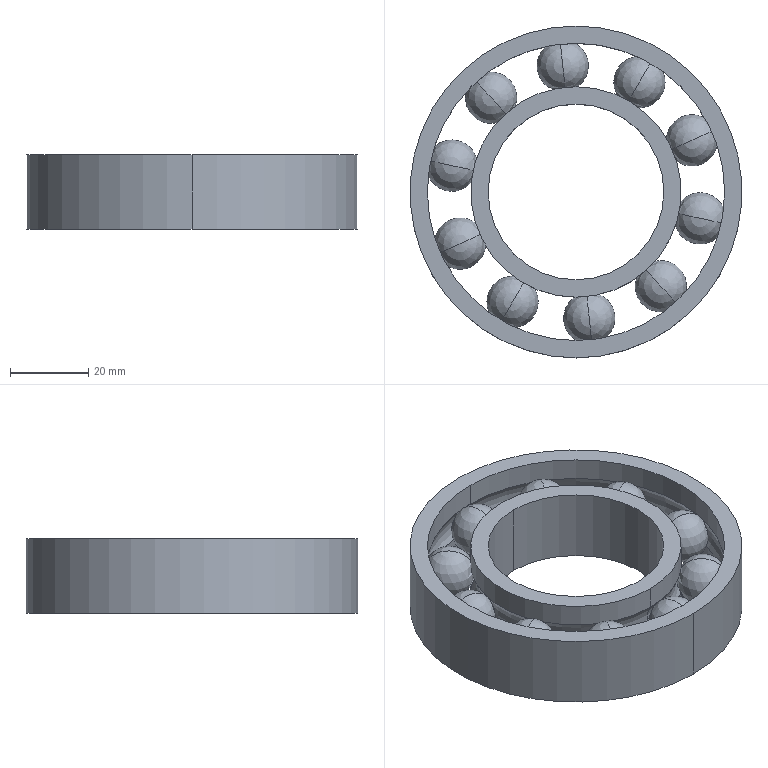Part | NX | features BREP 12 | 12 solids | 40 faces | box 85 x 85 x 19 mm | volume 44629 mm3 | sphere 20 | cylinder 12 | torus 4 | plane 4 | commonest cylinder face diameters 53.889 x4 76.111 x4 45 x2 85 x2
STEP:
#1=CARTESIAN_POINT('',(29.69,13.219,6.667));
#2=VERTEX_POINT('',#1);
#3=CARTESIAN_POINT('',(29.69,13.219,-6.667));
#4=VERTEX_POINT('',#3);
#5=CARTESIAN_POINT('',(29.69,13.219,0.));
#6=DIRECTION('',(-0.4067,0.9135,0.));
#7=DIRECTION('',(0.,0.,-1.));
#8=AXIS2_PLACEMENT_3D('',#5,#6,#7);
#9=CIRCLE('',#8,6.667);
#10=EDGE_CURVE('',#2,#4,#9,.F.);
#11=ORIENTED_EDGE('',*,*,#10,.T.);
#12=CARTESIAN_POINT('',(29.69,13.219,0.));
#13=DIRECTION('',(0.4067,-0.9135,0.));
#14=DIRECTION('',(0.,0.,-1.));
#15=AXIS2_PLACEMENT_3D('',#12,#13,#14);
#16=CIRCLE('',#15,6.667);
#17=EDGE_CURVE('',#2,#4,#16,.F.);
#18=ORIENTED_EDGE('',*,*,#17,.F.);
#19=EDGE_LOOP('',(#11,#18));
#20=FACE_BOUND('',#19,.T.);
#21=CARTESIAN_POINT('',(29.69,13.219,0.));
#22=DIRECTION('',(0.,0.,-1.));
#23=DIRECTION('',(0.9135,0.4067,0.));
#24=AXIS2_PLACEMENT_3D('',#21,#22,#23);
#25=SPHERICAL_SURFACE('',#24,6.667);
#26=ADVANCED_FACE('',(#20),#25,.T.);
#27=ORIENTED_EDGE('',*,*,#10,.F.);
#28=ORIENTED_EDGE('',*,*,#17,.T.);
#29=EDGE_LOOP('',(#27,#28));
#30=FACE_BOUND('',#29,.T.);
#31=CARTESIAN_POINT('',(29.69,13.219,0.));
#32=DIRECTION('',(0.,0.,-1.));
#33=DIRECTION('',(0.9135,0.4067,0.));
#34=AXIS2_PLACEMENT_3D('',#31,#32,#33);
#35=SPHERICAL_SURFACE('',#34,6.667);
#36=ADVANCED_FACE('',(#30),#35,.T.);
#37=CLOSED_SHELL('',(#26,#36));
#38=MANIFOLD_SOLID_BREP('',#37);
#39=CARTESIAN_POINT('',(31.79,-6.757,6.667));
#40=VERTEX_POINT('',#39);
#41=CARTESIAN_POINT('',(31.79,-6.757,-6.667));
#42=VERTEX_POINT('',#41);
#43=CARTESIAN_POINT('',(31.79,-6.757,0.));
#44=DIRECTION('',(0.2079,0.9781,0.));
#45=DIRECTION('',(0.,0.,-1.));
#46=AXIS2_PLACEMENT_3D('',#43,#44,#45);
#47=CIRCLE('',#46,6.667);
#48=EDGE_CURVE('',#40,#42,#47,.F.);
#49=ORIENTED_EDGE('',*,*,#48,.T.);
#50=CARTESIAN_POINT('',(31.79,-6.757,0.));
#51=DIRECTION('',(-0.2079,-0.9781,0.));
#52=DIRECTION('',(0.,0.,-1.));
#53=AXIS2_PLACEMENT_3D('',#50,#51,#52);
#54=CIRCLE('',#53,6.667);
#55=EDGE_CURVE('',#40,#42,#54,.F.);
#56=ORIENTED_EDGE('',*,*,#55,.F.);
#57=EDGE_LOOP('',(#49,#56));
#58=FACE_BOUND('',#57,.T.);
#59=CARTESIAN_POINT('',(31.79,-6.757,0.));
#60=DIRECTION('',(0.,0.,-1.));
#61=DIRECTION('',(0.9781,-0.2079,0.));
#62=AXIS2_PLACEMENT_3D('',#59,#60,#61);
#63=SPHERICAL_SURFACE('',#62,6.667);
#64=ADVANCED_FACE('',(#58),#63,.T.);
#65=ORIENTED_EDGE('',*,*,#48,.F.);
#66=ORIENTED_EDGE('',*,*,#55,.T.);
#67=EDGE_LOOP('',(#65,#66));
#68=FACE_BOUND('',#67,.T.);
#69=CARTESIAN_POINT('',(31.79,-6.757,0.));
#70=DIRECTION('',(0.,0.,-1.));
#71=DIRECTION('',(0.9781,-0.2079,0.));
#72=AXIS2_PLACEMENT_3D('',#69,#70,#71);
#73=SPHERICAL_SURFACE('',#72,6.667);
#74=ADVANCED_FACE('',(#68),#73,.T.);
#75=CLOSED_SHELL('',(#64,#74));
#76=MANIFOLD_SOLID_BREP('',#75);
#77=CARTESIAN_POINT('',(-16.25,-28.146,-6.667));
#78=VERTEX_POINT('',#77);
#79=CARTESIAN_POINT('',(-16.25,-28.146,6.667));
#80=VERTEX_POINT('',#79);
#81=CARTESIAN_POINT('',(-16.25,-28.146,0.));
#82=DIRECTION('',(0.866,-0.5,0.));
#83=DIRECTION('',(0.,0.,-1.));
#84=AXIS2_PLACEMENT_3D('',#81,#82,#83);
#85=CIRCLE('',#84,6.667);
#86=EDGE_CURVE('',#78,#80,#85,.T.);
#87=ORIENTED_EDGE('',*,*,#86,.F.);
#88=CARTESIAN_POINT('',(-16.25,-28.146,0.));
#89=DIRECTION('',(-0.866,0.5,0.));
#90=DIRECTION('',(0.,0.,-1.));
#91=AXIS2_PLACEMENT_3D('',#88,#89,#90);
#92=CIRCLE('',#91,6.667);
#93=EDGE_CURVE('',#78,#80,#92,.T.);
#94=ORIENTED_EDGE('',*,*,#93,.T.);
#95=EDGE_LOOP('',(#87,#94));
#96=FACE_BOUND('',#95,.T.);
#97=CARTESIAN_POINT('',(-16.25,-28.146,0.));
#98=DIRECTION('',(0.,0.,-1.));
#99=DIRECTION('',(-0.5,-0.866,0.));
#100=AXIS2_PLACEMENT_3D('',#97,#98,#99);
#101=SPHERICAL_SURFACE('',#100,6.667);
#102=ADVANCED_FACE('',(#96),#101,.T.);
#103=ORIENTED_EDGE('',*,*,#86,.T.);
#104=ORIENTED_EDGE('',*,*,#93,.F.);
#105=EDGE_LOOP('',(#103,#104));
#106=FACE_BOUND('',#105,.T.);
#107=CARTESIAN_POINT('',(-16.25,-28.146,0.));
#108=DIRECTION('',(0.,0.,-1.));
#109=DIRECTION('',(-0.5,-0.866,0.));
#110=AXIS2_PLACEMENT_3D('',#107,#108,#109);
#111=SPHERICAL_SURFACE('',#110,6.667);
#112=ADVANCED_FACE('',(#106),#111,.T.);
#113=CLOSED_SHELL('',(#102,#112));
#114=MANIFOLD_SOLID_BREP('',#113);
#115=CARTESIAN_POINT('',(16.25,28.146,6.667));
#116=VERTEX_POINT('',#115);
#117=CARTESIAN_POINT('',(16.25,28.146,-6.667));
#118=VERTEX_POINT('',#117);
#119=CARTESIAN_POINT('',(16.25,28.146,0.));
#120=DIRECTION('',(-0.866,0.5,0.));
#121=DIRECTION('',(0.,0.,-1.));
#122=AXIS2_PLACEMENT_3D('',#119,#120,#121);
#123=CIRCLE('',#122,6.667);
#124=EDGE_CURVE('',#116,#118,#123,.F.);
#125=ORIENTED_EDGE('',*,*,#124,.T.);
#126=CARTESIAN_POINT('',(16.25,28.146,0.));
#127=DIRECTION('',(0.866,-0.5,0.));
#128=DIRECTION('',(0.,0.,-1.));
#129=AXIS2_PLACEMENT_3D('',#126,#127,#128);
#130=CIRCLE('',#129,6.667);
#131=EDGE_CURVE('',#116,#118,#130,.F.);
#132=ORIENTED_EDGE('',*,*,#131,.F.);
#133=EDGE_LOOP('',(#125,#132));
#134=FACE_BOUND('',#133,.T.);
#135=CARTESIAN_POINT('',(16.25,28.146,0.));
#136=DIRECTION('',(0.,0.,-1.));
#137=DIRECTION('',(0.5,0.866,0.));
#138=AXIS2_PLACEMENT_3D('',#135,#136,#137);
#139=SPHERICAL_SURFACE('',#138,6.667);
#140=ADVANCED_FACE('',(#134),#139,.T.);
#141=ORIENTED_EDGE('',*,*,#124,.F.);
#142=ORIENTED_EDGE('',*,*,#131,.T.);
#143=EDGE_LOOP('',(#141,#142));
#144=FACE_BOUND('',#143,.T.);
#145=CARTESIAN_POINT('',(16.25,28.146,0.));
#146=DIRECTION('',(0.,0.,-1.));
#147=DIRECTION('',(0.5,0.866,0.));
#148=AXIS2_PLACEMENT_3D('',#145,#146,#147);
#149=SPHERICAL_SURFACE('',#148,6.667);
#150=ADVANCED_FACE('',(#144),#149,.T.);
#151=CLOSED_SHELL('',(#140,#150));
#152=MANIFOLD_SOLID_BREP('',#151);
#153=CARTESIAN_POINT('',(-31.79,6.757,-6.667));
#154=VERTEX_POINT('',#153);
#155=CARTESIAN_POINT('',(-31.79,6.757,6.667));
#156=VERTEX_POINT('',#155);
#157=CARTESIAN_POINT('',(-31.79,6.757,0.));
#158=DIRECTION('',(-0.2079,-0.9781,0.));
#159=DIRECTION('',(0.,0.,-1.));
#160=AXIS2_PLACEMENT_3D('',#157,#158,#159);
#161=CIRCLE('',#160,6.667);
#162=EDGE_CURVE('',#154,#156,#161,.T.);
#163=ORIENTED_EDGE('',*,*,#162,.F.);
#164=CARTESIAN_POINT('',(-31.79,6.757,0.));
#165=DIRECTION('',(0.2079,0.9781,0.));
#166=DIRECTION('',(0.,0.,-1.));
#167=AXIS2_PLACEMENT_3D('',#164,#165,#166);
#168=CIRCLE('',#167,6.667);
#169=EDGE_CURVE('',#154,#156,#168,.T.);
#170=ORIENTED_EDGE('',*,*,#169,.T.);
#171=EDGE_LOOP('',(#163,#170));
#172=FACE_BOUND('',#171,.T.);
#173=CARTESIAN_POINT('',(-31.79,6.757,0.));
#174=DIRECTION('',(0.,0.,-1.));
#175=DIRECTION('',(-0.9781,0.2079,0.));
#176=AXIS2_PLACEMENT_3D('',#173,#174,#175);
#177=SPHERICAL_SURFACE('',#176,6.667);
#178=ADVANCED_FACE('',(#172),#177,.T.);
#179=ORIENTED_EDGE('',*,*,#162,.T.);
#180=ORIENTED_EDGE('',*,*,#169,.F.);
#181=EDGE_LOOP('',(#179,#180));
#182=FACE_BOUND('',#181,.T.);
#183=CARTESIAN_POINT('',(-31.79,6.757,0.));
#184=DIRECTION('',(0.,0.,-1.));
#185=DIRECTION('',(-0.9781,0.2079,0.));
#186=AXIS2_PLACEMENT_3D('',#183,#184,#185);
#187=SPHERICAL_SURFACE('',#186,6.667);
#188=ADVANCED_FACE('',(#182),#187,.T.);
#189=CLOSED_SHELL('',(#178,#188));
#190=MANIFOLD_SOLID_BREP('',#189);
#191=CARTESIAN_POINT('',(3.397,-32.322,6.667));
#192=VERTEX_POINT('',#191);
#193=CARTESIAN_POINT('',(3.397,-32.322,-6.667));
#194=VERTEX_POINT('',#193);
#195=CARTESIAN_POINT('',(3.397,-32.322,0.));
#196=DIRECTION('',(0.9945,0.1045,0.));
#197=DIRECTION('',(0.,0.,-1.));
#198=AXIS2_PLACEMENT_3D('',#195,#196,#197);
#199=CIRCLE('',#198,6.667);
#200=EDGE_CURVE('',#192,#194,#199,.F.);
#201=ORIENTED_EDGE('',*,*,#200,.T.);
#202=CARTESIAN_POINT('',(3.397,-32.322,0.));
#203=DIRECTION('',(-0.9945,-0.1045,0.));
#204=DIRECTION('',(0.,0.,-1.));
#205=AXIS2_PLACEMENT_3D('',#202,#203,#204);
#206=CIRCLE('',#205,6.667);
#207=EDGE_CURVE('',#192,#194,#206,.F.);
#208=ORIENTED_EDGE('',*,*,#207,.F.);
#209=EDGE_LOOP('',(#201,#208));
#210=FACE_BOUND('',#209,.T.);
#211=CARTESIAN_POINT('',(3.397,-32.322,0.));
#212=DIRECTION('',(0.,0.,-1.));
#213=DIRECTION('',(0.1045,-0.9945,0.));
#214=AXIS2_PLACEMENT_3D('',#211,#212,#213);
#215=SPHERICAL_SURFACE('',#214,6.667);
#216=ADVANCED_FACE('',(#210),#215,.T.);
#217=ORIENTED_EDGE('',*,*,#200,.F.);
#218=ORIENTED_EDGE('',*,*,#207,.T.);
#219=EDGE_LOOP('',(#217,#218));
#220=FACE_BOUND('',#219,.T.);
#221=CARTESIAN_POINT('',(3.397,-32.322,0.));
#222=DIRECTION('',(0.,0.,-1.));
#223=DIRECTION('',(0.1045,-0.9945,0.));
#224=AXIS2_PLACEMENT_3D('',#221,#222,#223);
#225=SPHERICAL_SURFACE('',#224,6.667);
#226=ADVANCED_FACE('',(#220),#225,.T.);
#227=CLOSED_SHELL('',(#216,#226));
#228=MANIFOLD_SOLID_BREP('',#227);
#229=CARTESIAN_POINT('',(-29.69,-13.219,-6.667));
#230=VERTEX_POINT('',#229);
#231=CARTESIAN_POINT('',(-29.69,-13.219,6.667));
#232=VERTEX_POINT('',#231);
#233=CARTESIAN_POINT('',(-29.69,-13.219,0.));
#234=DIRECTION('',(0.4067,-0.9135,0.));
#235=DIRECTION('',(0.,0.,-1.));
#236=AXIS2_PLACEMENT_3D('',#233,#234,#235);
#237=CIRCLE('',#236,6.667);
#238=EDGE_CURVE('',#230,#232,#237,.T.);
#239=ORIENTED_EDGE('',*,*,#238,.F.);
#240=CARTESIAN_POINT('',(-29.69,-13.219,0.));
#241=DIRECTION('',(-0.4067,0.9135,0.));
#242=DIRECTION('',(0.,0.,-1.));
#243=AXIS2_PLACEMENT_3D('',#240,#241,#242);
#244=CIRCLE('',#243,6.667);
#245=EDGE_CURVE('',#230,#232,#244,.T.);
#246=ORIENTED_EDGE('',*,*,#245,.T.);
#247=EDGE_LOOP('',(#239,#246));
#248=FACE_BOUND('',#247,.T.);
#249=CARTESIAN_POINT('',(-29.69,-13.219,0.));
#250=DIRECTION('',(0.,0.,-1.));
#251=DIRECTION('',(-0.9135,-0.4067,0.));
#252=AXIS2_PLACEMENT_3D('',#249,#250,#251);
#253=SPHERICAL_SURFACE('',#252,6.667);
#254=ADVANCED_FACE('',(#248),#253,.T.);
#255=ORIENTED_EDGE('',*,*,#238,.T.);
#256=ORIENTED_EDGE('',*,*,#245,.F.);
#257=EDGE_LOOP('',(#255,#256));
#258=FACE_BOUND('',#257,.T.);
#259=CARTESIAN_POINT('',(-29.69,-13.219,0.));
#260=DIRECTION('',(0.,0.,-1.));
#261=DIRECTION('',(-0.9135,-0.4067,0.));
#262=AXIS2_PLACEMENT_3D('',#259,#260,#261);
#263=SPHERICAL_SURFACE('',#262,6.667);
#264=ADVANCED_FACE('',(#258),#263,.T.);
#265=CLOSED_SHELL('',(#254,#264));
#266=MANIFOLD_SOLID_BREP('',#265);
#267=CARTESIAN_POINT('',(-21.747,24.152,-6.667));
#268=VERTEX_POINT('',#267);
#269=CARTESIAN_POINT('',(-21.747,24.152,6.667));
#270=VERTEX_POINT('',#269);
#271=CARTESIAN_POINT('',(-21.747,24.152,0.));
#272=DIRECTION('',(-0.7431,-0.6691,0.));
#273=DIRECTION('',(0.,0.,-1.));
#274=AXIS2_PLACEMENT_3D('',#271,#272,#273);
#275=CIRCLE('',#274,6.667);
#276=EDGE_CURVE('',#268,#270,#275,.T.);
#277=ORIENTED_EDGE('',*,*,#276,.F.);
#278=CARTESIAN_POINT('',(-21.747,24.152,0.));
#279=DIRECTION('',(0.7431,0.6691,0.));
#280=DIRECTION('',(0.,0.,-1.));
#281=AXIS2_PLACEMENT_3D('',#278,#279,#280);
#282=CIRCLE('',#281,6.667);
#283=EDGE_CURVE('',#268,#270,#282,.T.);
#284=ORIENTED_EDGE('',*,*,#283,.T.);
#285=EDGE_LOOP('',(#277,#284));
#286=FACE_BOUND('',#285,.T.);
#287=CARTESIAN_POINT('',(-21.747,24.152,0.));
#288=DIRECTION('',(0.,0.,-1.));
#289=DIRECTION('',(-0.6691,0.7431,0.));
#290=AXIS2_PLACEMENT_3D('',#287,#288,#289);
#291=SPHERICAL_SURFACE('',#290,6.667);
#292=ADVANCED_FACE('',(#286),#291,.T.);
#293=ORIENTED_EDGE('',*,*,#276,.T.);
#294=ORIENTED_EDGE('',*,*,#283,.F.);
#295=EDGE_LOOP('',(#293,#294));
#296=FACE_BOUND('',#295,.T.);
#297=CARTESIAN_POINT('',(-21.747,24.152,0.));
#298=DIRECTION('',(0.,0.,-1.));
#299=DIRECTION('',(-0.6691,0.7431,0.));
#300=AXIS2_PLACEMENT_3D('',#297,#298,#299);
#301=SPHERICAL_SURFACE('',#300,6.667);
#302=ADVANCED_FACE('',(#296),#301,.T.);
#303=CLOSED_SHELL('',(#292,#302));
#304=MANIFOLD_SOLID_BREP('',#303);
#305=CARTESIAN_POINT('',(0.,26.944,3.685));
#306=VERTEX_POINT('',#305);
#307=CARTESIAN_POINT('',(0.,-26.944,3.685));
#308=VERTEX_POINT('',#307);
#309=CARTESIAN_POINT('',(0.,0.,3.685));
#310=DIRECTION('',(0.,0.,1.));
#311=DIRECTION('',(0.,1.,0.));
#312=AXIS2_PLACEMENT_3D('',#309,#310,#311);
#313=CIRCLE('',#312,26.944);
#314=EDGE_CURVE('',#306,#308,#313,.T.);
#315=ORIENTED_EDGE('',*,*,#314,.T.);
#316=CARTESIAN_POINT('',(0.,-26.944,9.5));
#317=VERTEX_POINT('',#316);
#318=CARTESIAN_POINT('',(0.,-26.944,3.685));
#319=DIRECTION('',(0.,0.,1.));
#320=VECTOR('',#319,1000.);
#321=LINE('',#318,#320);
#322=EDGE_CURVE('',#308,#317,#321,.T.);
#323=ORIENTED_EDGE('',*,*,#322,.T.);
#324=CARTESIAN_POINT('',(0.,26.944,9.5));
#325=VERTEX_POINT('',#324);
#326=CARTESIAN_POINT('',(0.,0.,9.5));
#327=DIRECTION('',(0.,0.,1.));
#328=DIRECTION('',(0.,1.,0.));
#329=AXIS2_PLACEMENT_3D('',#326,#327,#328);
#330=CIRCLE('',#329,26.944);
#331=EDGE_CURVE('',#325,#317,#330,.T.);
#332=ORIENTED_EDGE('',*,*,#331,.F.);
#333=CARTESIAN_POINT('',(0.,26.944,3.685));
#334=DIRECTION('',(0.,0.,1.));
#335=VECTOR('',#334,1000.);
#336=LINE('',#333,#335);
#337=EDGE_CURVE('',#306,#325,#336,.T.);
#338=ORIENTED_EDGE('',*,*,#337,.F.);
#339=EDGE_LOOP('',(#315,#323,#332,#338));
#340=FACE_BOUND('',#339,.T.);
#341=CARTESIAN_POINT('',(0.,0.,10.45));
#342=DIRECTION('',(0.,0.,-1.));
#343=DIRECTION('',(0.,1.,0.));
#344=AXIS2_PLACEMENT_3D('',#341,#342,#343);
#345=CYLINDRICAL_SURFACE('',#344,26.944);
#346=ADVANCED_FACE('',(#340),#345,.T.);
#347=CARTESIAN_POINT('',(0.,0.,9.5));
#348=DIRECTION('',(0.,0.,-1.));
#349=DIRECTION('',(0.,1.,0.));
#350=AXIS2_PLACEMENT_3D('',#347,#348,#349);
#351=CIRCLE('',#350,26.944);
#352=EDGE_CURVE('',#325,#317,#351,.T.);
#353=ORIENTED_EDGE('',*,*,#352,.T.);
#354=ORIENTED_EDGE('',*,*,#322,.F.);
#355=CARTESIAN_POINT('',(0.,0.,3.685));
#356=DIRECTION('',(0.,0.,-1.));
#357=DIRECTION('',(0.,1.,0.));
#358=AXIS2_PLACEMENT_3D('',#355,#356,#357);
#359=CIRCLE('',#358,26.944);
#360=EDGE_CURVE('',#306,#308,#359,.T.);
#361=ORIENTED_EDGE('',*,*,#360,.F.);
#362=ORIENTED_EDGE('',*,*,#337,.T.);
#363=EDGE_LOOP('',(#353,#354,#361,#362));
#364=FACE_BOUND('',#363,.T.);
#365=CARTESIAN_POINT('',(0.,0.,10.45));
#366=DIRECTION('',(0.,0.,-1.));
#367=DIRECTION('',(0.,1.,0.));
#368=AXIS2_PLACEMENT_3D('',#365,#366,#367);
#369=CYLINDRICAL_SURFACE('',#368,26.944);
#370=ADVANCED_FACE('',(#364),#369,.T.);
#371=ORIENTED_EDGE('',*,*,#360,.T.);
#372=CARTESIAN_POINT('',(0.,-26.944,-3.685));
#373=VERTEX_POINT('',#372);
#374=CARTESIAN_POINT('',(0.,-32.5,0.));
#375=DIRECTION('',(1.,0.,0.));
#376=DIRECTION('',(0.,0.8333,-0.5528));
#377=AXIS2_PLACEMENT_3D('',#374,#375,#376);
#378=CIRCLE('',#377,6.667);
#379=EDGE_CURVE('',#308,#373,#378,.F.);
#380=ORIENTED_EDGE('',*,*,#379,.T.);
#381=CARTESIAN_POINT('',(0.,26.944,-3.685));
#382=VERTEX_POINT('',#381);
#383=CARTESIAN_POINT('',(0.,0.,-3.685));
#384=DIRECTION('',(0.,0.,-1.));
#385=DIRECTION('',(0.,1.,0.));
#386=AXIS2_PLACEMENT_3D('',#383,#384,#385);
#387=CIRCLE('',#386,26.944);
#388=EDGE_CURVE('',#382,#373,#387,.T.);
#389=ORIENTED_EDGE('',*,*,#388,.F.);
#390=CARTESIAN_POINT('',(0.,32.5,0.));
#391=DIRECTION('',(-1.,0.,0.));
#392=DIRECTION('',(0.,-0.8333,-0.5528));
#393=AXIS2_PLACEMENT_3D('',#390,#391,#392);
#394=CIRCLE('',#393,6.667);
#395=EDGE_CURVE('',#306,#382,#394,.F.);
#396=ORIENTED_EDGE('',*,*,#395,.F.);
#397=EDGE_LOOP('',(#371,#380,#389,#396));
#398=FACE_BOUND('',#397,.T.);
#399=CARTESIAN_POINT('',(0.,0.,0.));
#400=DIRECTION('',(0.,0.,-1.));
#401=DIRECTION('',(0.,1.,0.));
#402=AXIS2_PLACEMENT_3D('',#399,#400,#401);
#403=TOROIDAL_SURFACE('',#402,32.5,6.667);
#404=ADVANCED_FACE('',(#398),#403,.F.);
#405=CARTESIAN_POINT('',(0.,0.,-3.685));
#406=DIRECTION('',(0.,0.,1.));
#407=DIRECTION('',(0.,1.,0.));
#408=AXIS2_PLACEMENT_3D('',#405,#406,#407);
#409=CIRCLE('',#408,26.944);
#410=EDGE_CURVE('',#382,#373,#409,.T.);
#411=ORIENTED_EDGE('',*,*,#410,.T.);
#412=ORIENTED_EDGE('',*,*,#379,.F.);
#413=ORIENTED_EDGE('',*,*,#314,.F.);
#414=ORIENTED_EDGE('',*,*,#395,.T.);
#415=EDGE_LOOP('',(#411,#412,#413,#414));
#416=FACE_BOUND('',#415,.T.);
#417=CARTESIAN_POINT('',(0.,0.,0.));
#418=DIRECTION('',(0.,0.,-1.));
#419=DIRECTION('',(0.,1.,0.));
#420=AXIS2_PLACEMENT_3D('',#417,#418,#419);
#421=TOROIDAL_SURFACE('',#420,32.5,6.667);
#422=ADVANCED_FACE('',(#416),#421,.F.);
#423=CARTESIAN_POINT('',(0.,26.944,-9.5));
#424=VERTEX_POINT('',#423);
#425=CARTESIAN_POINT('',(0.,-26.944,-9.5));
#426=VERTEX_POINT('',#425);
#427=CARTESIAN_POINT('',(0.,0.,-9.5));
#428=DIRECTION('',(0.,0.,1.));
#429=DIRECTION('',(0.,1.,0.));
#430=AXIS2_PLACEMENT_3D('',#427,#428,#429);
#431=CIRCLE('',#430,26.944);
#432=EDGE_CURVE('',#424,#426,#431,.T.);
#433=ORIENTED_EDGE('',*,*,#432,.T.);
#434=CARTESIAN_POINT('',(0.,-26.944,-9.5));
#435=DIRECTION('',(0.,0.,1.));
#436=VECTOR('',#435,1000.);
#437=LINE('',#434,#436);
#438=EDGE_CURVE('',#426,#373,#437,.T.);
#439=ORIENTED_EDGE('',*,*,#438,.T.);
#440=ORIENTED_EDGE('',*,*,#410,.F.);
#441=CARTESIAN_POINT('',(0.,26.944,-9.5));
#442=DIRECTION('',(0.,0.,1.));
#443=VECTOR('',#442,1000.);
#444=LINE('',#441,#443);
#445=EDGE_CURVE('',#424,#382,#444,.T.);
#446=ORIENTED_EDGE('',*,*,#445,.F.);
#447=EDGE_LOOP('',(#433,#439,#440,#446));
#448=FACE_BOUND('',#447,.T.);
#449=CARTESIAN_POINT('',(0.,0.,10.45));
#450=DIRECTION('',(0.,0.,-1.));
#451=DIRECTION('',(0.,1.,0.));
#452=AXIS2_PLACEMENT_3D('',#449,#450,#451);
#453=CYLINDRICAL_SURFACE('',#452,26.944);
#454=ADVANCED_FACE('',(#448),#453,.T.);
#455=ORIENTED_EDGE('',*,*,#388,.T.);
#456=ORIENTED_EDGE('',*,*,#438,.F.);
#457=CARTESIAN_POINT('',(0.,0.,-9.5));
#458=DIRECTION('',(0.,0.,-1.));
#459=DIRECTION('',(0.,1.,0.));
#460=AXIS2_PLACEMENT_3D('',#457,#458,#459);
#461=CIRCLE('',#460,26.944);
#462=EDGE_CURVE('',#424,#426,#461,.T.);
#463=ORIENTED_EDGE('',*,*,#462,.F.);
#464=ORIENTED_EDGE('',*,*,#445,.T.);
#465=EDGE_LOOP('',(#455,#456,#463,#464));
#466=FACE_BOUND('',#465,.T.);
#467=CARTESIAN_POINT('',(0.,0.,10.45));
#468=DIRECTION('',(0.,0.,-1.));
#469=DIRECTION('',(0.,1.,0.));
#470=AXIS2_PLACEMENT_3D('',#467,#468,#469);
#471=CYLINDRICAL_SURFACE('',#470,26.944);
#472=ADVANCED_FACE('',(#466),#471,.T.);
#473=ORIENTED_EDGE('',*,*,#432,.F.);
#474=ORIENTED_EDGE('',*,*,#462,.T.);
#475=EDGE_LOOP('',(#473,#474));
#476=FACE_BOUND('',#475,.T.);
#477=CARTESIAN_POINT('',(0.,22.5,-9.5));
#478=VERTEX_POINT('',#477);
#479=CARTESIAN_POINT('',(0.,-22.5,-9.5));
#480=VERTEX_POINT('',#479);
#481=CARTESIAN_POINT('',(0.,0.,-9.5));
#482=DIRECTION('',(0.,0.,-1.));
#483=DIRECTION('',(0.,1.,0.));
#484=AXIS2_PLACEMENT_3D('',#481,#482,#483);
#485=CIRCLE('',#484,22.5);
#486=EDGE_CURVE('',#478,#480,#485,.T.);
#487=ORIENTED_EDGE('',*,*,#486,.F.);
#488=CARTESIAN_POINT('',(0.,0.,-9.5));
#489=DIRECTION('',(0.,0.,1.));
#490=DIRECTION('',(0.,1.,0.));
#491=AXIS2_PLACEMENT_3D('',#488,#489,#490);
#492=CIRCLE('',#491,22.5);
#493=EDGE_CURVE('',#478,#480,#492,.T.);
#494=ORIENTED_EDGE('',*,*,#493,.T.);
#495=EDGE_LOOP('',(#487,#494));
#496=FACE_BOUND('',#495,.T.);
#497=CARTESIAN_POINT('',(0.,0.,-9.5));
#498=DIRECTION('',(0.,0.,-1.));
#499=DIRECTION('',(0.,1.,0.));
#500=AXIS2_PLACEMENT_3D('',#497,#498,#499);
#501=PLANE('',#500);
#502=ADVANCED_FACE('',(#476,#496),#501,.T.);
#503=CARTESIAN_POINT('',(0.,22.5,9.5));
#504=VERTEX_POINT('',#503);
#505=CARTESIAN_POINT('',(0.,-22.5,9.5));
#506=VERTEX_POINT('',#505);
#507=CARTESIAN_POINT('',(0.,0.,9.5));
#508=DIRECTION('',(0.,0.,1.));
#509=DIRECTION('',(0.,1.,0.));
#510=AXIS2_PLACEMENT_3D('',#507,#508,#509);
#511=CIRCLE('',#510,22.5);
#512=EDGE_CURVE('',#504,#506,#511,.T.);
#513=ORIENTED_EDGE('',*,*,#512,.T.);
#514=CARTESIAN_POINT('',(0.,-22.5,9.5));
#515=DIRECTION('',(0.,0.,-1.));
#516=VECTOR('',#515,1000.);
#517=LINE('',#514,#516);
#518=EDGE_CURVE('',#506,#480,#517,.T.);
#519=ORIENTED_EDGE('',*,*,#518,.T.);
#520=ORIENTED_EDGE('',*,*,#493,.F.);
#521=CARTESIAN_POINT('',(0.,22.5,9.5));
#522=DIRECTION('',(0.,0.,-1.));
#523=VECTOR('',#522,1000.);
#524=LINE('',#521,#523);
#525=EDGE_CURVE('',#504,#478,#524,.T.);
#526=ORIENTED_EDGE('',*,*,#525,.F.);
#527=EDGE_LOOP('',(#513,#519,#520,#526));
#528=FACE_BOUND('',#527,.T.);
#529=CARTESIAN_POINT('',(0.,0.,10.45));
#530=DIRECTION('',(0.,0.,-1.));
#531=DIRECTION('',(0.,1.,0.));
#532=AXIS2_PLACEMENT_3D('',#529,#530,#531);
#533=CYLINDRICAL_SURFACE('',#532,22.5);
#534=ADVANCED_FACE('',(#528),#533,.F.);
#535=ORIENTED_EDGE('',*,*,#486,.T.);
#536=ORIENTED_EDGE('',*,*,#518,.F.);
#537=CARTESIAN_POINT('',(0.,0.,9.5));
#538=DIRECTION('',(0.,0.,-1.));
#539=DIRECTION('',(0.,1.,0.));
#540=AXIS2_PLACEMENT_3D('',#537,#538,#539);
#541=CIRCLE('',#540,22.5);
#542=EDGE_CURVE('',#504,#506,#541,.T.);
#543=ORIENTED_EDGE('',*,*,#542,.F.);
#544=ORIENTED_EDGE('',*,*,#525,.T.);
#545=EDGE_LOOP('',(#535,#536,#543,#544));
#546=FACE_BOUND('',#545,.T.);
#547=CARTESIAN_POINT('',(0.,0.,10.45));
#548=DIRECTION('',(0.,0.,-1.));
#549=DIRECTION('',(0.,1.,0.));
#550=AXIS2_PLACEMENT_3D('',#547,#548,#549);
#551=CYLINDRICAL_SURFACE('',#550,22.5);
#552=ADVANCED_FACE('',(#546),#551,.F.);
#553=ORIENTED_EDGE('',*,*,#352,.F.);
#554=ORIENTED_EDGE('',*,*,#331,.T.);
#555=EDGE_LOOP('',(#553,#554));
#556=FACE_BOUND('',#555,.T.);
#557=ORIENTED_EDGE('',*,*,#512,.F.);
#558=ORIENTED_EDGE('',*,*,#542,.T.);
#559=EDGE_LOOP('',(#557,#558));
#560=FACE_BOUND('',#559,.T.);
#561=CARTESIAN_POINT('',(0.,0.,9.5));
#562=DIRECTION('',(0.,0.,-1.));
#563=DIRECTION('',(0.,1.,0.));
#564=AXIS2_PLACEMENT_3D('',#561,#562,#563);
#565=PLANE('',#564);
#566=ADVANCED_FACE('',(#556,#560),#565,.F.);
#567=CLOSED_SHELL('',(#346,#370,#404,#422,#454,#472,#502,#534,#552,#566));
#568=MANIFOLD_SOLID_BREP('',#567);
#569=CARTESIAN_POINT('',(-3.397,32.322,-6.667));
#570=VERTEX_POINT('',#569);
#571=CARTESIAN_POINT('',(-3.397,32.322,6.667));
#572=VERTEX_POINT('',#571);
#573=CARTESIAN_POINT('',(-3.397,32.322,0.));
#574=DIRECTION('',(-0.9945,-0.1045,0.));
#575=DIRECTION('',(0.,0.,-1.));
#576=AXIS2_PLACEMENT_3D('',#573,#574,#575);
#577=CIRCLE('',#576,6.667);
#578=EDGE_CURVE('',#570,#572,#577,.T.);
#579=ORIENTED_EDGE('',*,*,#578,.F.);
#580=CARTESIAN_POINT('',(-3.397,32.322,0.));
#581=DIRECTION('',(0.9945,0.1045,0.));
#582=DIRECTION('',(0.,0.,-1.));
#583=AXIS2_PLACEMENT_3D('',#580,#581,#582);
#584=CIRCLE('',#583,6.667);
#585=EDGE_CURVE('',#570,#572,#584,.T.);
#586=ORIENTED_EDGE('',*,*,#585,.T.);
#587=EDGE_LOOP('',(#579,#586));
#588=FACE_BOUND('',#587,.T.);
#589=CARTESIAN_POINT('',(-3.397,32.322,0.));
#590=DIRECTION('',(0.,0.,-1.));
#591=DIRECTION('',(-0.1045,0.9945,0.));
#592=AXIS2_PLACEMENT_3D('',#589,#590,#591);
#593=SPHERICAL_SURFACE('',#592,6.667);
#594=ADVANCED_FACE('',(#588),#593,.T.);
#595=ORIENTED_EDGE('',*,*,#578,.T.);
#596=ORIENTED_EDGE('',*,*,#585,.F.);
#597=EDGE_LOOP('',(#595,#596));
#598=FACE_BOUND('',#597,.T.);
#599=CARTESIAN_POINT('',(-3.397,32.322,0.));
#600=DIRECTION('',(0.,0.,-1.));
#601=DIRECTION('',(-0.1045,0.9945,0.));
#602=AXIS2_PLACEMENT_3D('',#599,#600,#601);
#603=SPHERICAL_SURFACE('',#602,6.667);
#604=ADVANCED_FACE('',(#598),#603,.T.);
#605=CLOSED_SHELL('',(#594,#604));
#606=MANIFOLD_SOLID_BREP('',#605);
#607=CARTESIAN_POINT('',(21.747,-24.152,6.667));
#608=VERTEX_POINT('',#607);
#609=CARTESIAN_POINT('',(21.747,-24.152,-6.667));
#610=VERTEX_POINT('',#609);
#611=CARTESIAN_POINT('',(21.747,-24.152,0.));
#612=DIRECTION('',(0.7431,0.6691,0.));
#613=DIRECTION('',(0.,0.,-1.));
#614=AXIS2_PLACEMENT_3D('',#611,#612,#613);
#615=CIRCLE('',#614,6.667);
#616=EDGE_CURVE('',#608,#610,#615,.F.);
#617=ORIENTED_EDGE('',*,*,#616,.T.);
#618=CARTESIAN_POINT('',(21.747,-24.152,0.));
#619=DIRECTION('',(-0.7431,-0.6691,0.));
#620=DIRECTION('',(0.,0.,-1.));
#621=AXIS2_PLACEMENT_3D('',#618,#619,#620);
#622=CIRCLE('',#621,6.667);
#623=EDGE_CURVE('',#608,#610,#622,.F.);
#624=ORIENTED_EDGE('',*,*,#623,.F.);
#625=EDGE_LOOP('',(#617,#624));
#626=FACE_BOUND('',#625,.T.);
#627=CARTESIAN_POINT('',(21.747,-24.152,0.));
#628=DIRECTION('',(0.,0.,-1.));
#629=DIRECTION('',(0.6691,-0.7431,0.));
#630=AXIS2_PLACEMENT_3D('',#627,#628,#629);
#631=SPHERICAL_SURFACE('',#630,6.667);
#632=ADVANCED_FACE('',(#626),#631,.T.);
#633=ORIENTED_EDGE('',*,*,#616,.F.);
#634=ORIENTED_EDGE('',*,*,#623,.T.);
#635=EDGE_LOOP('',(#633,#634));
#636=FACE_BOUND('',#635,.T.);
#637=CARTESIAN_POINT('',(21.747,-24.152,0.));
#638=DIRECTION('',(0.,0.,-1.));
#639=DIRECTION('',(0.6691,-0.7431,0.));
#640=AXIS2_PLACEMENT_3D('',#637,#638,#639);
#641=SPHERICAL_SURFACE('',#640,6.667);
#642=ADVANCED_FACE('',(#636),#641,.T.);
#643=CLOSED_SHELL('',(#632,#642));
#644=MANIFOLD_SOLID_BREP('',#643);
#645=CARTESIAN_POINT('',(0.,42.5,-9.5));
#646=VERTEX_POINT('',#645);
#647=CARTESIAN_POINT('',(0.,-42.5,-9.5));
#648=VERTEX_POINT('',#647);
#649=CARTESIAN_POINT('',(0.,0.,-9.5));
#650=DIRECTION('',(0.,0.,1.));
#651=DIRECTION('',(0.,1.,0.));
#652=AXIS2_PLACEMENT_3D('',#649,#650,#651);
#653=CIRCLE('',#652,42.5);
#654=EDGE_CURVE('',#646,#648,#653,.T.);
#655=ORIENTED_EDGE('',*,*,#654,.T.);
#656=CARTESIAN_POINT('',(0.,-42.5,9.5));
#657=VERTEX_POINT('',#656);
#658=CARTESIAN_POINT('',(0.,-42.5,-9.5));
#659=DIRECTION('',(0.,0.,1.));
#660=VECTOR('',#659,1000.);
#661=LINE('',#658,#660);
#662=EDGE_CURVE('',#648,#657,#661,.T.);
#663=ORIENTED_EDGE('',*,*,#662,.T.);
#664=CARTESIAN_POINT('',(0.,42.5,9.5));
#665=VERTEX_POINT('',#664);
#666=CARTESIAN_POINT('',(0.,0.,9.5));
#667=DIRECTION('',(0.,0.,1.));
#668=DIRECTION('',(0.,1.,0.));
#669=AXIS2_PLACEMENT_3D('',#666,#667,#668);
#670=CIRCLE('',#669,42.5);
#671=EDGE_CURVE('',#665,#657,#670,.T.);
#672=ORIENTED_EDGE('',*,*,#671,.F.);
#673=CARTESIAN_POINT('',(0.,42.5,-9.5));
#674=DIRECTION('',(0.,0.,1.));
#675=VECTOR('',#674,1000.);
#676=LINE('',#673,#675);
#677=EDGE_CURVE('',#646,#665,#676,.T.);
#678=ORIENTED_EDGE('',*,*,#677,.F.);
#679=EDGE_LOOP('',(#655,#663,#672,#678));
#680=FACE_BOUND('',#679,.T.);
#681=CARTESIAN_POINT('',(0.,0.,10.45));
#682=DIRECTION('',(0.,0.,-1.));
#683=DIRECTION('',(0.,1.,0.));
#684=AXIS2_PLACEMENT_3D('',#681,#682,#683);
#685=CYLINDRICAL_SURFACE('',#684,42.5);
#686=ADVANCED_FACE('',(#680),#685,.T.);
#687=CARTESIAN_POINT('',(0.,0.,9.5));
#688=DIRECTION('',(0.,0.,-1.));
#689=DIRECTION('',(0.,1.,0.));
#690=AXIS2_PLACEMENT_3D('',#687,#688,#689);
#691=CIRCLE('',#690,42.5);
#692=EDGE_CURVE('',#665,#657,#691,.T.);
#693=ORIENTED_EDGE('',*,*,#692,.T.);
#694=ORIENTED_EDGE('',*,*,#662,.F.);
#695=CARTESIAN_POINT('',(0.,0.,-9.5));
#696=DIRECTION('',(0.,0.,-1.));
#697=DIRECTION('',(0.,1.,0.));
#698=AXIS2_PLACEMENT_3D('',#695,#696,#697);
#699=CIRCLE('',#698,42.5);
#700=EDGE_CURVE('',#646,#648,#699,.T.);
#701=ORIENTED_EDGE('',*,*,#700,.F.);
#702=ORIENTED_EDGE('',*,*,#677,.T.);
#703=EDGE_LOOP('',(#693,#694,#701,#702));
#704=FACE_BOUND('',#703,.T.);
#705=CARTESIAN_POINT('',(0.,0.,10.45));
#706=DIRECTION('',(0.,0.,-1.));
#707=DIRECTION('',(0.,1.,0.));
#708=AXIS2_PLACEMENT_3D('',#705,#706,#707);
#709=CYLINDRICAL_SURFACE('',#708,42.5);
#710=ADVANCED_FACE('',(#704),#709,.T.);
#711=ORIENTED_EDGE('',*,*,#654,.F.);
#712=ORIENTED_EDGE('',*,*,#700,.T.);
#713=EDGE_LOOP('',(#711,#712));
#714=FACE_BOUND('',#713,.T.);
#715=CARTESIAN_POINT('',(0.,38.056,-9.5));
#716=VERTEX_POINT('',#715);
#717=CARTESIAN_POINT('',(0.,-38.056,-9.5));
#718=VERTEX_POINT('',#717);
#719=CARTESIAN_POINT('',(0.,0.,-9.5));
#720=DIRECTION('',(0.,0.,-1.));
#721=DIRECTION('',(0.,1.,0.));
#722=AXIS2_PLACEMENT_3D('',#719,#720,#721);
#723=CIRCLE('',#722,38.056);
#724=EDGE_CURVE('',#716,#718,#723,.T.);
#725=ORIENTED_EDGE('',*,*,#724,.F.);
#726=CARTESIAN_POINT('',(0.,0.,-9.5));
#727=DIRECTION('',(0.,0.,1.));
#728=DIRECTION('',(0.,1.,0.));
#729=AXIS2_PLACEMENT_3D('',#726,#727,#728);
#730=CIRCLE('',#729,38.056);
#731=EDGE_CURVE('',#716,#718,#730,.T.);
#732=ORIENTED_EDGE('',*,*,#731,.T.);
#733=EDGE_LOOP('',(#725,#732));
#734=FACE_BOUND('',#733,.T.);
#735=CARTESIAN_POINT('',(0.,0.,-9.5));
#736=DIRECTION('',(0.,0.,-1.));
#737=DIRECTION('',(0.,1.,0.));
#738=AXIS2_PLACEMENT_3D('',#735,#736,#737);
#739=PLANE('',#738);
#740=ADVANCED_FACE('',(#714,#734),#739,.T.);
#741=CARTESIAN_POINT('',(0.,38.056,-3.685));
#742=VERTEX_POINT('',#741);
#743=CARTESIAN_POINT('',(0.,-38.056,-3.685));
#744=VERTEX_POINT('',#743);
#745=CARTESIAN_POINT('',(0.,0.,-3.685));
#746=DIRECTION('',(0.,0.,1.));
#747=DIRECTION('',(0.,1.,0.));
#748=AXIS2_PLACEMENT_3D('',#745,#746,#747);
#749=CIRCLE('',#748,38.056);
#750=EDGE_CURVE('',#742,#744,#749,.T.);
#751=ORIENTED_EDGE('',*,*,#750,.T.);
#752=CARTESIAN_POINT('',(0.,-38.056,-3.685));
#753=DIRECTION('',(0.,0.,-1.));
#754=VECTOR('',#753,1000.);
#755=LINE('',#752,#754);
#756=EDGE_CURVE('',#744,#718,#755,.T.);
#757=ORIENTED_EDGE('',*,*,#756,.T.);
#758=ORIENTED_EDGE('',*,*,#731,.F.);
#759=CARTESIAN_POINT('',(0.,38.056,-3.685));
#760=DIRECTION('',(0.,0.,-1.));
#761=VECTOR('',#760,1000.);
#762=LINE('',#759,#761);
#763=EDGE_CURVE('',#742,#716,#762,.T.);
#764=ORIENTED_EDGE('',*,*,#763,.F.);
#765=EDGE_LOOP('',(#751,#757,#758,#764));
#766=FACE_BOUND('',#765,.T.);
#767=CARTESIAN_POINT('',(0.,0.,10.45));
#768=DIRECTION('',(0.,0.,-1.));
#769=DIRECTION('',(0.,1.,0.));
#770=AXIS2_PLACEMENT_3D('',#767,#768,#769);
#771=CYLINDRICAL_SURFACE('',#770,38.056);
#772=ADVANCED_FACE('',(#766),#771,.F.);
#773=ORIENTED_EDGE('',*,*,#724,.T.);
#774=ORIENTED_EDGE('',*,*,#756,.F.);
#775=CARTESIAN_POINT('',(0.,0.,-3.685));
#776=DIRECTION('',(0.,0.,-1.));
#777=DIRECTION('',(0.,1.,0.));
#778=AXIS2_PLACEMENT_3D('',#775,#776,#777);
#779=CIRCLE('',#778,38.056);
#780=EDGE_CURVE('',#742,#744,#779,.T.);
#781=ORIENTED_EDGE('',*,*,#780,.F.);
#782=ORIENTED_EDGE('',*,*,#763,.T.);
#783=EDGE_LOOP('',(#773,#774,#781,#782));
#784=FACE_BOUND('',#783,.T.);
#785=CARTESIAN_POINT('',(0.,0.,10.45));
#786=DIRECTION('',(0.,0.,-1.));
#787=DIRECTION('',(0.,1.,0.));
#788=AXIS2_PLACEMENT_3D('',#785,#786,#787);
#789=CYLINDRICAL_SURFACE('',#788,38.056);
#790=ADVANCED_FACE('',(#784),#789,.F.);
#791=ORIENTED_EDGE('',*,*,#780,.T.);
#792=CARTESIAN_POINT('',(0.,-38.056,3.685));
#793=VERTEX_POINT('',#792);
#794=CARTESIAN_POINT('',(0.,-32.5,0.));
#795=DIRECTION('',(1.,0.,0.));
#796=DIRECTION('',(0.,-0.8333,0.5528));
#797=AXIS2_PLACEMENT_3D('',#794,#795,#796);
#798=CIRCLE('',#797,6.667);
#799=EDGE_CURVE('',#744,#793,#798,.F.);
#800=ORIENTED_EDGE('',*,*,#799,.T.);
#801=CARTESIAN_POINT('',(0.,38.056,3.685));
#802=VERTEX_POINT('',#801);
#803=CARTESIAN_POINT('',(0.,0.,3.685));
#804=DIRECTION('',(0.,0.,-1.));
#805=DIRECTION('',(0.,1.,0.));
#806=AXIS2_PLACEMENT_3D('',#803,#804,#805);
#807=CIRCLE('',#806,38.056);
#808=EDGE_CURVE('',#802,#793,#807,.T.);
#809=ORIENTED_EDGE('',*,*,#808,.F.);
#810=CARTESIAN_POINT('',(0.,32.5,0.));
#811=DIRECTION('',(-1.,0.,0.));
#812=DIRECTION('',(0.,0.8333,0.5528));
#813=AXIS2_PLACEMENT_3D('',#810,#811,#812);
#814=CIRCLE('',#813,6.667);
#815=EDGE_CURVE('',#742,#802,#814,.F.);
#816=ORIENTED_EDGE('',*,*,#815,.F.);
#817=EDGE_LOOP('',(#791,#800,#809,#816));
#818=FACE_BOUND('',#817,.T.);
#819=CARTESIAN_POINT('',(0.,0.,0.));
#820=DIRECTION('',(0.,0.,-1.));
#821=DIRECTION('',(0.,1.,0.));
#822=AXIS2_PLACEMENT_3D('',#819,#820,#821);
#823=TOROIDAL_SURFACE('',#822,32.5,6.667);
#824=ADVANCED_FACE('',(#818),#823,.F.);
#825=CARTESIAN_POINT('',(0.,0.,3.685));
#826=DIRECTION('',(0.,0.,1.));
#827=DIRECTION('',(0.,1.,0.));
#828=AXIS2_PLACEMENT_3D('',#825,#826,#827);
#829=CIRCLE('',#828,38.056);
#830=EDGE_CURVE('',#802,#793,#829,.T.);
#831=ORIENTED_EDGE('',*,*,#830,.T.);
#832=ORIENTED_EDGE('',*,*,#799,.F.);
#833=ORIENTED_EDGE('',*,*,#750,.F.);
#834=ORIENTED_EDGE('',*,*,#815,.T.);
#835=EDGE_LOOP('',(#831,#832,#833,#834));
#836=FACE_BOUND('',#835,.T.);
#837=CARTESIAN_POINT('',(0.,0.,0.));
#838=DIRECTION('',(0.,0.,-1.));
#839=DIRECTION('',(0.,1.,0.));
#840=AXIS2_PLACEMENT_3D('',#837,#838,#839);
#841=TOROIDAL_SURFACE('',#840,32.5,6.667);
#842=ADVANCED_FACE('',(#836),#841,.F.);
#843=CARTESIAN_POINT('',(0.,38.056,9.5));
#844=VERTEX_POINT('',#843);
#845=CARTESIAN_POINT('',(0.,-38.056,9.5));
#846=VERTEX_POINT('',#845);
#847=CARTESIAN_POINT('',(0.,0.,9.5));
#848=DIRECTION('',(0.,0.,1.));
#849=DIRECTION('',(0.,1.,0.));
#850=AXIS2_PLACEMENT_3D('',#847,#848,#849);
#851=CIRCLE('',#850,38.056);
#852=EDGE_CURVE('',#844,#846,#851,.T.);
#853=ORIENTED_EDGE('',*,*,#852,.T.);
#854=CARTESIAN_POINT('',(0.,-38.056,9.5));
#855=DIRECTION('',(0.,0.,-1.));
#856=VECTOR('',#855,1000.);
#857=LINE('',#854,#856);
#858=EDGE_CURVE('',#846,#793,#857,.T.);
#859=ORIENTED_EDGE('',*,*,#858,.T.);
#860=ORIENTED_EDGE('',*,*,#830,.F.);
#861=CARTESIAN_POINT('',(0.,38.056,9.5));
#862=DIRECTION('',(0.,0.,-1.));
#863=VECTOR('',#862,1000.);
#864=LINE('',#861,#863);
#865=EDGE_CURVE('',#844,#802,#864,.T.);
#866=ORIENTED_EDGE('',*,*,#865,.F.);
#867=EDGE_LOOP('',(#853,#859,#860,#866));
#868=FACE_BOUND('',#867,.T.);
#869=CARTESIAN_POINT('',(0.,0.,10.45));
#870=DIRECTION('',(0.,0.,-1.));
#871=DIRECTION('',(0.,1.,0.));
#872=AXIS2_PLACEMENT_3D('',#869,#870,#871);
#873=CYLINDRICAL_SURFACE('',#872,38.056);
#874=ADVANCED_FACE('',(#868),#873,.F.);
#875=ORIENTED_EDGE('',*,*,#808,.T.);
#876=ORIENTED_EDGE('',*,*,#858,.F.);
#877=CARTESIAN_POINT('',(0.,0.,9.5));
#878=DIRECTION('',(0.,0.,-1.));
#879=DIRECTION('',(0.,1.,0.));
#880=AXIS2_PLACEMENT_3D('',#877,#878,#879);
#881=CIRCLE('',#880,38.056);
#882=EDGE_CURVE('',#844,#846,#881,.T.);
#883=ORIENTED_EDGE('',*,*,#882,.F.);
#884=ORIENTED_EDGE('',*,*,#865,.T.);
#885=EDGE_LOOP('',(#875,#876,#883,#884));
#886=FACE_BOUND('',#885,.T.);
#887=CARTESIAN_POINT('',(0.,0.,10.45));
#888=DIRECTION('',(0.,0.,-1.));
#889=DIRECTION('',(0.,1.,0.));
#890=AXIS2_PLACEMENT_3D('',#887,#888,#889);
#891=CYLINDRICAL_SURFACE('',#890,38.056);
#892=ADVANCED_FACE('',(#886),#891,.F.);
#893=ORIENTED_EDGE('',*,*,#692,.F.);
#894=ORIENTED_EDGE('',*,*,#671,.T.);
#895=EDGE_LOOP('',(#893,#894));
#896=FACE_BOUND('',#895,.T.);
#897=ORIENTED_EDGE('',*,*,#852,.F.);
#898=ORIENTED_EDGE('',*,*,#882,.T.);
#899=EDGE_LOOP('',(#897,#898));
#900=FACE_BOUND('',#899,.T.);
#901=CARTESIAN_POINT('',(0.,0.,9.5));
#902=DIRECTION('',(0.,0.,-1.));
#903=DIRECTION('',(0.,1.,0.));
#904=AXIS2_PLACEMENT_3D('',#901,#902,#903);
#905=PLANE('',#904);
#906=ADVANCED_FACE('',(#896,#900),#905,.F.);
#907=CLOSED_SHELL('',(#686,#710,#740,#772,#790,#824,#842,#874,#892,#906));
#908=MANIFOLD_SOLID_BREP('',#907);
#909=(LENGTH_UNIT()NAMED_UNIT(*)SI_UNIT(.MILLI.,.METRE.));
#910=UNCERTAINTY_MEASURE_WITH_UNIT(LENGTH_MEASURE(0.00001),#909,'','');
#911=(NAMED_UNIT(*)PLANE_ANGLE_UNIT()SI_UNIT($,.RADIAN.));
#912=(NAMED_UNIT(*)SI_UNIT($,.STERADIAN.)SOLID_ANGLE_UNIT());
#913=(GEOMETRIC_REPRESENTATION_CONTEXT(3)GLOBAL_UNCERTAINTY_ASSIGNED_CONTEXT((#910))GLOBAL_UNIT_ASSIGNED_CONTEXT((#909,#911,#912))REPRESENTATION_CONTEXT('',''));
#914=ADVANCED_BREP_SHAPE_REPRESENTATION('',(#38,#76,#114,#152,#190,#228,#266,#304,#568,#606,#644,#908),#913);